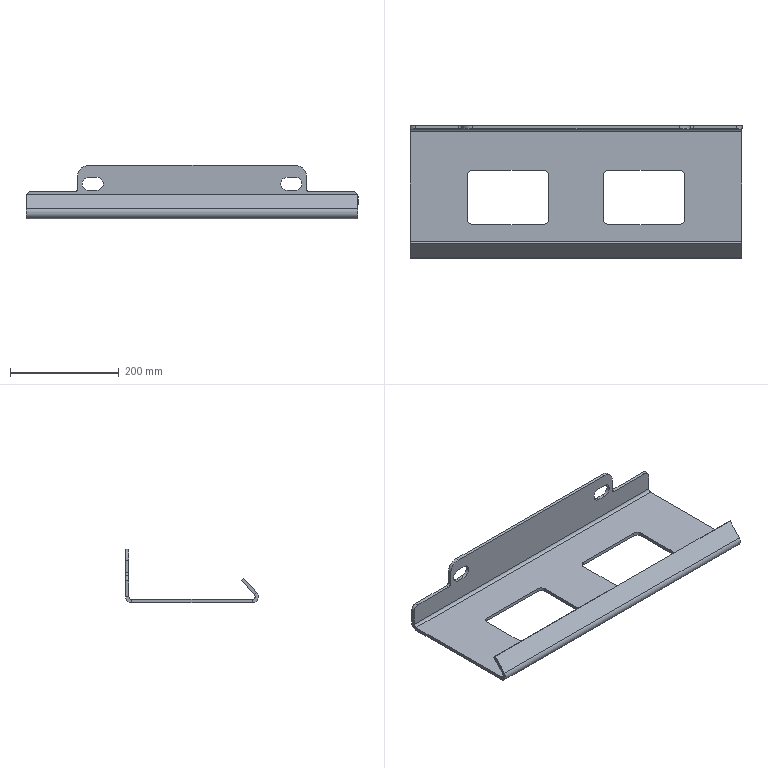Part | SolidWorks | features SM3dBend 2, FlatPattern 1, SMBaseFlange 1, SheetMetal 1 | 1 solid | 60 faces | box 610 x 243.695 x 98.004 mm | volume 1127789 mm3 | plane 34 | cylinder 26 | commonest cylinder face diameters 20 x12 24 x6 10 x4 22 x2 40 x2